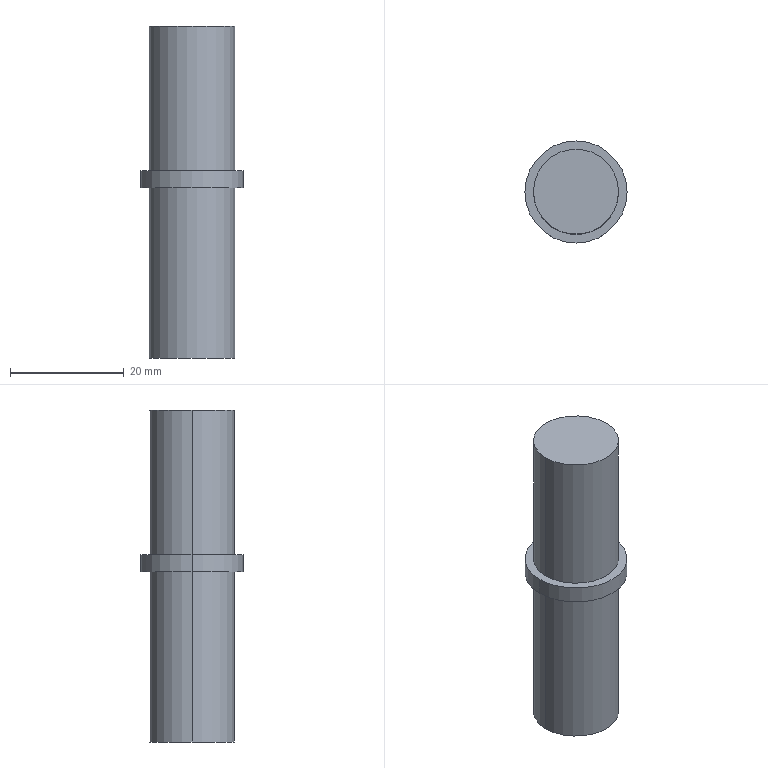Part | SolidWorks | features ICE 4, Extrusion 1 | 1 solid | 10 faces | box 18 x 18 x 58.5 mm | volume 10571 mm3 | cylinder 6 | plane 4 | commonest cylinder face diameters 15 x4 18 x2
STEP:
#1=CARTESIAN_POINT('',(7.5,0.,100.));
#2=VERTEX_POINT('',#1);
#3=CARTESIAN_POINT('',(-7.5,0.,100.));
#4=VERTEX_POINT('',#3);
#5=CARTESIAN_POINT('',(0.,0.,100.));
#6=DIRECTION('',(0.,0.,1.));
#7=DIRECTION('',(1.,0.,0.));
#8=AXIS2_PLACEMENT_3D('',#5,#6,#7);
#9=CIRCLE('',#8,7.5);
#10=EDGE_CURVE('',#2,#4,#9,.T.);
#11=ORIENTED_EDGE('',*,*,#10,.F.);
#12=CARTESIAN_POINT('',(7.5,0.,74.5));
#13=VERTEX_POINT('',#12);
#14=CARTESIAN_POINT('',(7.5,0.,100.));
#15=DIRECTION('',(0.,0.,-1.));
#16=VECTOR('',#15,1000.);
#17=LINE('',#14,#16);
#18=EDGE_CURVE('',#2,#13,#17,.T.);
#19=ORIENTED_EDGE('',*,*,#18,.T.);
#20=CARTESIAN_POINT('',(-7.5,0.,74.5));
#21=VERTEX_POINT('',#20);
#22=CARTESIAN_POINT('',(0.,0.,74.5));
#23=DIRECTION('',(0.,0.,1.));
#24=DIRECTION('',(1.,0.,0.));
#25=AXIS2_PLACEMENT_3D('',#22,#23,#24);
#26=CIRCLE('',#25,7.5);
#27=EDGE_CURVE('',#13,#21,#26,.T.);
#28=ORIENTED_EDGE('',*,*,#27,.T.);
#29=CARTESIAN_POINT('',(-7.5,0.,100.));
#30=DIRECTION('',(0.,0.,-1.));
#31=VECTOR('',#30,1000.);
#32=LINE('',#29,#31);
#33=EDGE_CURVE('',#4,#21,#32,.T.);
#34=ORIENTED_EDGE('',*,*,#33,.F.);
#35=EDGE_LOOP('',(#11,#19,#28,#34));
#36=FACE_OUTER_BOUND('',#35,.T.);
#37=CARTESIAN_POINT('',(0.,0.,100.));
#38=DIRECTION('',(0.,0.,-1.));
#39=DIRECTION('',(-1.,0.,0.));
#40=AXIS2_PLACEMENT_3D('',#37,#38,#39);
#41=CYLINDRICAL_SURFACE('',#40,7.5);
#42=ADVANCED_FACE('',(#36),#41,.T.);
#43=CARTESIAN_POINT('',(9.,0.,71.5));
#44=VERTEX_POINT('',#43);
#45=CARTESIAN_POINT('',(-9.,0.,71.5));
#46=VERTEX_POINT('',#45);
#47=CARTESIAN_POINT('',(0.,0.,71.5));
#48=DIRECTION('',(0.,0.,1.));
#49=DIRECTION('',(1.,0.,0.));
#50=AXIS2_PLACEMENT_3D('',#47,#48,#49);
#51=CIRCLE('',#50,9.);
#52=EDGE_CURVE('',#44,#46,#51,.T.);
#53=ORIENTED_EDGE('',*,*,#52,.T.);
#54=CARTESIAN_POINT('',(-9.,0.,74.5));
#55=VERTEX_POINT('',#54);
#56=CARTESIAN_POINT('',(-9.,0.,71.5));
#57=DIRECTION('',(0.,0.,1.));
#58=VECTOR('',#57,1000.);
#59=LINE('',#56,#58);
#60=EDGE_CURVE('',#46,#55,#59,.T.);
#61=ORIENTED_EDGE('',*,*,#60,.T.);
#62=CARTESIAN_POINT('',(9.,0.,74.5));
#63=VERTEX_POINT('',#62);
#64=CARTESIAN_POINT('',(0.,0.,74.5));
#65=DIRECTION('',(0.,0.,1.));
#66=DIRECTION('',(1.,0.,0.));
#67=AXIS2_PLACEMENT_3D('',#64,#65,#66);
#68=CIRCLE('',#67,9.);
#69=EDGE_CURVE('',#63,#55,#68,.T.);
#70=ORIENTED_EDGE('',*,*,#69,.F.);
#71=CARTESIAN_POINT('',(9.,0.,71.5));
#72=DIRECTION('',(0.,0.,1.));
#73=VECTOR('',#72,1000.);
#74=LINE('',#71,#73);
#75=EDGE_CURVE('',#44,#63,#74,.T.);
#76=ORIENTED_EDGE('',*,*,#75,.F.);
#77=EDGE_LOOP('',(#53,#61,#70,#76));
#78=FACE_OUTER_BOUND('',#77,.T.);
#79=CARTESIAN_POINT('',(0.,0.,71.5));
#80=DIRECTION('',(0.,0.,1.));
#81=DIRECTION('',(1.,0.,0.));
#82=AXIS2_PLACEMENT_3D('',#79,#80,#81);
#83=CYLINDRICAL_SURFACE('',#82,9.);
#84=ADVANCED_FACE('',(#78),#83,.T.);
#85=CARTESIAN_POINT('',(7.5,0.,71.5));
#86=VERTEX_POINT('',#85);
#87=CARTESIAN_POINT('',(-7.5,0.,71.5));
#88=VERTEX_POINT('',#87);
#89=CARTESIAN_POINT('',(0.,0.,71.5));
#90=DIRECTION('',(0.,0.,1.));
#91=DIRECTION('',(1.,0.,0.));
#92=AXIS2_PLACEMENT_3D('',#89,#90,#91);
#93=CIRCLE('',#92,7.5);
#94=EDGE_CURVE('',#86,#88,#93,.T.);
#95=ORIENTED_EDGE('',*,*,#94,.F.);
#96=CARTESIAN_POINT('',(7.5,0.,41.5));
#97=VERTEX_POINT('',#96);
#98=CARTESIAN_POINT('',(7.5,0.,100.));
#99=DIRECTION('',(0.,0.,-1.));
#100=VECTOR('',#99,1000.);
#101=LINE('',#98,#100);
#102=EDGE_CURVE('',#86,#97,#101,.T.);
#103=ORIENTED_EDGE('',*,*,#102,.T.);
#104=CARTESIAN_POINT('',(-7.5,0.,41.5));
#105=VERTEX_POINT('',#104);
#106=CARTESIAN_POINT('',(0.,0.,41.5));
#107=DIRECTION('',(0.,0.,-1.));
#108=DIRECTION('',(-1.,0.,0.));
#109=AXIS2_PLACEMENT_3D('',#106,#107,#108);
#110=CIRCLE('',#109,7.5);
#111=EDGE_CURVE('',#105,#97,#110,.T.);
#112=ORIENTED_EDGE('',*,*,#111,.F.);
#113=CARTESIAN_POINT('',(-7.5,0.,100.));
#114=DIRECTION('',(0.,0.,-1.));
#115=VECTOR('',#114,1000.);
#116=LINE('',#113,#115);
#117=EDGE_CURVE('',#88,#105,#116,.T.);
#118=ORIENTED_EDGE('',*,*,#117,.F.);
#119=EDGE_LOOP('',(#95,#103,#112,#118));
#120=FACE_OUTER_BOUND('',#119,.T.);
#121=CARTESIAN_POINT('',(0.,0.,100.));
#122=DIRECTION('',(0.,0.,-1.));
#123=DIRECTION('',(-1.,0.,0.));
#124=AXIS2_PLACEMENT_3D('',#121,#122,#123);
#125=CYLINDRICAL_SURFACE('',#124,7.5);
#126=ADVANCED_FACE('',(#120),#125,.T.);
#127=ORIENTED_EDGE('',*,*,#102,.F.);
#128=CARTESIAN_POINT('',(0.,0.,71.5));
#129=DIRECTION('',(0.,0.,1.));
#130=DIRECTION('',(1.,0.,0.));
#131=AXIS2_PLACEMENT_3D('',#128,#129,#130);
#132=CIRCLE('',#131,7.5);
#133=EDGE_CURVE('',#88,#86,#132,.T.);
#134=ORIENTED_EDGE('',*,*,#133,.F.);
#135=ORIENTED_EDGE('',*,*,#117,.T.);
#136=CARTESIAN_POINT('',(0.,0.,41.5));
#137=DIRECTION('',(0.,0.,-1.));
#138=DIRECTION('',(-1.,0.,0.));
#139=AXIS2_PLACEMENT_3D('',#136,#137,#138);
#140=CIRCLE('',#139,7.5);
#141=EDGE_CURVE('',#97,#105,#140,.T.);
#142=ORIENTED_EDGE('',*,*,#141,.F.);
#143=EDGE_LOOP('',(#127,#134,#135,#142));
#144=FACE_OUTER_BOUND('',#143,.T.);
#145=CARTESIAN_POINT('',(0.,0.,100.));
#146=DIRECTION('',(0.,0.,-1.));
#147=DIRECTION('',(-1.,0.,0.));
#148=AXIS2_PLACEMENT_3D('',#145,#146,#147);
#149=CYLINDRICAL_SURFACE('',#148,7.5);
#150=ADVANCED_FACE('',(#144),#149,.T.);
#151=ORIENTED_EDGE('',*,*,#60,.F.);
#152=CARTESIAN_POINT('',(0.,0.,71.5));
#153=DIRECTION('',(0.,0.,1.));
#154=DIRECTION('',(1.,0.,0.));
#155=AXIS2_PLACEMENT_3D('',#152,#153,#154);
#156=CIRCLE('',#155,9.);
#157=EDGE_CURVE('',#46,#44,#156,.T.);
#158=ORIENTED_EDGE('',*,*,#157,.T.);
#159=ORIENTED_EDGE('',*,*,#75,.T.);
#160=CARTESIAN_POINT('',(0.,0.,74.5));
#161=DIRECTION('',(0.,0.,1.));
#162=DIRECTION('',(1.,0.,0.));
#163=AXIS2_PLACEMENT_3D('',#160,#161,#162);
#164=CIRCLE('',#163,9.);
#165=EDGE_CURVE('',#55,#63,#164,.T.);
#166=ORIENTED_EDGE('',*,*,#165,.F.);
#167=EDGE_LOOP('',(#151,#158,#159,#166));
#168=FACE_OUTER_BOUND('',#167,.T.);
#169=CARTESIAN_POINT('',(0.,0.,71.5));
#170=DIRECTION('',(0.,0.,1.));
#171=DIRECTION('',(1.,0.,0.));
#172=AXIS2_PLACEMENT_3D('',#169,#170,#171);
#173=CYLINDRICAL_SURFACE('',#172,9.);
#174=ADVANCED_FACE('',(#168),#173,.T.);
#175=ORIENTED_EDGE('',*,*,#133,.T.);
#176=ORIENTED_EDGE('',*,*,#94,.T.);
#177=EDGE_LOOP('',(#175,#176));
#178=FACE_BOUND('',#177,.T.);
#179=ORIENTED_EDGE('',*,*,#52,.F.);
#180=ORIENTED_EDGE('',*,*,#157,.F.);
#181=EDGE_LOOP('',(#179,#180));
#182=FACE_OUTER_BOUND('',#181,.T.);
#183=CARTESIAN_POINT('',(0.,0.,71.5));
#184=DIRECTION('',(0.,0.,1.));
#185=DIRECTION('',(1.,0.,0.));
#186=AXIS2_PLACEMENT_3D('',#183,#184,#185);
#187=PLANE('',#186);
#188=ADVANCED_FACE('',(#178,#182),#187,.F.);
#189=CARTESIAN_POINT('',(0.,0.,74.5));
#190=DIRECTION('',(0.,0.,1.));
#191=DIRECTION('',(1.,0.,0.));
#192=AXIS2_PLACEMENT_3D('',#189,#190,#191);
#193=CIRCLE('',#192,7.5);
#194=EDGE_CURVE('',#21,#13,#193,.T.);
#195=ORIENTED_EDGE('',*,*,#194,.F.);
#196=ORIENTED_EDGE('',*,*,#27,.F.);
#197=EDGE_LOOP('',(#195,#196));
#198=FACE_BOUND('',#197,.T.);
#199=ORIENTED_EDGE('',*,*,#69,.T.);
#200=ORIENTED_EDGE('',*,*,#165,.T.);
#201=EDGE_LOOP('',(#199,#200));
#202=FACE_OUTER_BOUND('',#201,.T.);
#203=CARTESIAN_POINT('',(0.,0.,74.5));
#204=DIRECTION('',(0.,0.,1.));
#205=DIRECTION('',(1.,0.,0.));
#206=AXIS2_PLACEMENT_3D('',#203,#204,#205);
#207=PLANE('',#206);
#208=ADVANCED_FACE('',(#198,#202),#207,.T.);
#209=CARTESIAN_POINT('',(0.,0.,100.));
#210=DIRECTION('',(0.,0.,1.));
#211=DIRECTION('',(1.,0.,0.));
#212=AXIS2_PLACEMENT_3D('',#209,#210,#211);
#213=CIRCLE('',#212,7.5);
#214=EDGE_CURVE('',#4,#2,#213,.T.);
#215=ORIENTED_EDGE('',*,*,#214,.T.);
#216=ORIENTED_EDGE('',*,*,#10,.T.);
#217=EDGE_LOOP('',(#215,#216));
#218=FACE_OUTER_BOUND('',#217,.T.);
#219=CARTESIAN_POINT('',(0.,0.,100.));
#220=DIRECTION('',(0.,0.,1.));
#221=DIRECTION('',(1.,0.,0.));
#222=AXIS2_PLACEMENT_3D('',#219,#220,#221);
#223=PLANE('',#222);
#224=ADVANCED_FACE('',(#218),#223,.T.);
#225=ORIENTED_EDGE('',*,*,#18,.F.);
#226=ORIENTED_EDGE('',*,*,#214,.F.);
#227=ORIENTED_EDGE('',*,*,#33,.T.);
#228=ORIENTED_EDGE('',*,*,#194,.T.);
#229=EDGE_LOOP('',(#225,#226,#227,#228));
#230=FACE_OUTER_BOUND('',#229,.T.);
#231=CARTESIAN_POINT('',(0.,0.,100.));
#232=DIRECTION('',(0.,0.,-1.));
#233=DIRECTION('',(-1.,0.,0.));
#234=AXIS2_PLACEMENT_3D('',#231,#232,#233);
#235=CYLINDRICAL_SURFACE('',#234,7.5);
#236=ADVANCED_FACE('',(#230),#235,.T.);
#237=ORIENTED_EDGE('',*,*,#111,.T.);
#238=ORIENTED_EDGE('',*,*,#141,.T.);
#239=EDGE_LOOP('',(#237,#238));
#240=FACE_OUTER_BOUND('',#239,.T.);
#241=CARTESIAN_POINT('',(0.,0.,41.5));
#242=DIRECTION('',(0.,0.,-1.));
#243=DIRECTION('',(-1.,0.,0.));
#244=AXIS2_PLACEMENT_3D('',#241,#242,#243);
#245=PLANE('',#244);
#246=ADVANCED_FACE('',(#240),#245,.T.);
#247=CLOSED_SHELL('',(#42,#84,#126,#150,#174,#188,#208,#224,#236,#246));
#248=MANIFOLD_SOLID_BREP('',#247);
#249=CARTESIAN_POINT('',(0.,0.,0.));
#250=DIRECTION('',(0.,0.,1.));
#251=DIRECTION('',(1.,0.,0.));
#252=AXIS2_PLACEMENT_3D('',#249,#250,#251);
#253=(LENGTH_UNIT()NAMED_UNIT(*)SI_UNIT(.MILLI.,.METRE.));
#254=UNCERTAINTY_MEASURE_WITH_UNIT(LENGTH_MEASURE(0.00001),#253,'','');
#255=(NAMED_UNIT(*)PLANE_ANGLE_UNIT()SI_UNIT($,.RADIAN.));
#256=(NAMED_UNIT(*)SI_UNIT($,.STERADIAN.)SOLID_ANGLE_UNIT());
#257=(GEOMETRIC_REPRESENTATION_CONTEXT(3)GLOBAL_UNCERTAINTY_ASSIGNED_CONTEXT((#254))GLOBAL_UNIT_ASSIGNED_CONTEXT((#253,#255,#256))REPRESENTATION_CONTEXT('',''));
#258=ADVANCED_BREP_SHAPE_REPRESENTATION('',(#248,#252),#257);